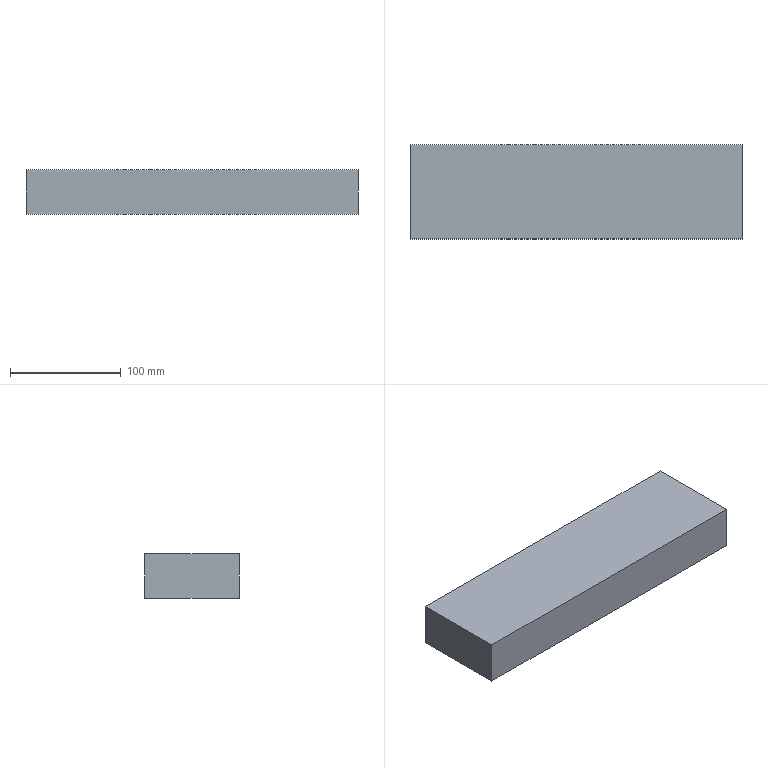Part | NX | features BREP 1 | 1 solid | 6 faces | box 300 x 85 x 40 mm | volume 1020000 mm3 | plane 6
STEP:
#1=CARTESIAN_POINT('',(-150.,42.5,-20.));
#2=VERTEX_POINT('',#1);
#3=CARTESIAN_POINT('',(-150.,-42.5,-20.));
#4=VERTEX_POINT('',#3);
#5=CARTESIAN_POINT('',(-150.,42.5,-20.));
#6=DIRECTION('',(0.,-1.,0.));
#7=VECTOR('',#6,1000.);
#8=LINE('',#5,#7);
#9=EDGE_CURVE('',#2,#4,#8,.T.);
#10=ORIENTED_EDGE('',*,*,#9,.T.);
#11=CARTESIAN_POINT('',(-150.,-42.5,20.));
#12=VERTEX_POINT('',#11);
#13=CARTESIAN_POINT('',(-150.,-42.5,20.));
#14=DIRECTION('',(0.,0.,-1.));
#15=VECTOR('',#14,1000.);
#16=LINE('',#13,#15);
#17=EDGE_CURVE('',#12,#4,#16,.T.);
#18=ORIENTED_EDGE('',*,*,#17,.F.);
#19=CARTESIAN_POINT('',(-150.,42.5,20.));
#20=VERTEX_POINT('',#19);
#21=CARTESIAN_POINT('',(-150.,42.5,20.));
#22=DIRECTION('',(0.,-1.,0.));
#23=VECTOR('',#22,1000.);
#24=LINE('',#21,#23);
#25=EDGE_CURVE('',#20,#12,#24,.T.);
#26=ORIENTED_EDGE('',*,*,#25,.F.);
#27=CARTESIAN_POINT('',(-150.,42.5,20.));
#28=DIRECTION('',(0.,0.,-1.));
#29=VECTOR('',#28,1000.);
#30=LINE('',#27,#29);
#31=EDGE_CURVE('',#20,#2,#30,.T.);
#32=ORIENTED_EDGE('',*,*,#31,.T.);
#33=EDGE_LOOP('',(#10,#18,#26,#32));
#34=FACE_BOUND('',#33,.T.);
#35=CARTESIAN_POINT('',(-150.,42.5,20.));
#36=DIRECTION('',(1.,0.,0.));
#37=DIRECTION('',(0.,0.,1.));
#38=AXIS2_PLACEMENT_3D('',#35,#36,#37);
#39=PLANE('',#38);
#40=ADVANCED_FACE('',(#34),#39,.F.);
#41=CARTESIAN_POINT('',(150.,-42.5,-20.));
#42=VERTEX_POINT('',#41);
#43=CARTESIAN_POINT('',(-150.,-42.5,-20.));
#44=DIRECTION('',(1.,0.,0.));
#45=VECTOR('',#44,1000.);
#46=LINE('',#43,#45);
#47=EDGE_CURVE('',#4,#42,#46,.T.);
#48=ORIENTED_EDGE('',*,*,#47,.T.);
#49=CARTESIAN_POINT('',(150.,-42.5,20.));
#50=VERTEX_POINT('',#49);
#51=CARTESIAN_POINT('',(150.,-42.5,20.));
#52=DIRECTION('',(0.,0.,-1.));
#53=VECTOR('',#52,1000.);
#54=LINE('',#51,#53);
#55=EDGE_CURVE('',#50,#42,#54,.T.);
#56=ORIENTED_EDGE('',*,*,#55,.F.);
#57=CARTESIAN_POINT('',(-150.,-42.5,20.));
#58=DIRECTION('',(1.,0.,0.));
#59=VECTOR('',#58,1000.);
#60=LINE('',#57,#59);
#61=EDGE_CURVE('',#12,#50,#60,.T.);
#62=ORIENTED_EDGE('',*,*,#61,.F.);
#63=ORIENTED_EDGE('',*,*,#17,.T.);
#64=EDGE_LOOP('',(#48,#56,#62,#63));
#65=FACE_BOUND('',#64,.T.);
#66=CARTESIAN_POINT('',(-150.,-42.5,20.));
#67=DIRECTION('',(0.,1.,0.));
#68=DIRECTION('',(0.,0.,-1.));
#69=AXIS2_PLACEMENT_3D('',#66,#67,#68);
#70=PLANE('',#69);
#71=ADVANCED_FACE('',(#65),#70,.F.);
#72=CARTESIAN_POINT('',(150.,42.5,-20.));
#73=VERTEX_POINT('',#72);
#74=CARTESIAN_POINT('',(150.,42.5,-20.));
#75=DIRECTION('',(0.,1.,0.));
#76=VECTOR('',#75,1000.);
#77=LINE('',#74,#76);
#78=EDGE_CURVE('',#42,#73,#77,.T.);
#79=ORIENTED_EDGE('',*,*,#78,.T.);
#80=CARTESIAN_POINT('',(150.,42.5,20.));
#81=VERTEX_POINT('',#80);
#82=CARTESIAN_POINT('',(150.,42.5,20.));
#83=DIRECTION('',(0.,0.,-1.));
#84=VECTOR('',#83,1000.);
#85=LINE('',#82,#84);
#86=EDGE_CURVE('',#81,#73,#85,.T.);
#87=ORIENTED_EDGE('',*,*,#86,.F.);
#88=CARTESIAN_POINT('',(150.,42.5,20.));
#89=DIRECTION('',(0.,1.,0.));
#90=VECTOR('',#89,1000.);
#91=LINE('',#88,#90);
#92=EDGE_CURVE('',#50,#81,#91,.T.);
#93=ORIENTED_EDGE('',*,*,#92,.F.);
#94=ORIENTED_EDGE('',*,*,#55,.T.);
#95=EDGE_LOOP('',(#79,#87,#93,#94));
#96=FACE_BOUND('',#95,.T.);
#97=CARTESIAN_POINT('',(150.,42.5,20.));
#98=DIRECTION('',(-1.,0.,0.));
#99=DIRECTION('',(0.,0.,-1.));
#100=AXIS2_PLACEMENT_3D('',#97,#98,#99);
#101=PLANE('',#100);
#102=ADVANCED_FACE('',(#96),#101,.F.);
#103=CARTESIAN_POINT('',(-150.,42.5,-20.));
#104=DIRECTION('',(-1.,0.,0.));
#105=VECTOR('',#104,1000.);
#106=LINE('',#103,#105);
#107=EDGE_CURVE('',#73,#2,#106,.T.);
#108=ORIENTED_EDGE('',*,*,#107,.T.);
#109=ORIENTED_EDGE('',*,*,#31,.F.);
#110=CARTESIAN_POINT('',(-150.,42.5,20.));
#111=DIRECTION('',(-1.,0.,0.));
#112=VECTOR('',#111,1000.);
#113=LINE('',#110,#112);
#114=EDGE_CURVE('',#81,#20,#113,.T.);
#115=ORIENTED_EDGE('',*,*,#114,.F.);
#116=ORIENTED_EDGE('',*,*,#86,.T.);
#117=EDGE_LOOP('',(#108,#109,#115,#116));
#118=FACE_BOUND('',#117,.T.);
#119=CARTESIAN_POINT('',(-150.,42.5,20.));
#120=DIRECTION('',(0.,-1.,0.));
#121=DIRECTION('',(0.,0.,1.));
#122=AXIS2_PLACEMENT_3D('',#119,#120,#121);
#123=PLANE('',#122);
#124=ADVANCED_FACE('',(#118),#123,.F.);
#125=ORIENTED_EDGE('',*,*,#25,.T.);
#126=ORIENTED_EDGE('',*,*,#61,.T.);
#127=ORIENTED_EDGE('',*,*,#92,.T.);
#128=ORIENTED_EDGE('',*,*,#114,.T.);
#129=EDGE_LOOP('',(#125,#126,#127,#128));
#130=FACE_BOUND('',#129,.T.);
#131=CARTESIAN_POINT('',(-150.,-42.5,20.));
#132=DIRECTION('',(0.,0.,1.));
#133=DIRECTION('',(-1.,0.,0.));
#134=AXIS2_PLACEMENT_3D('',#131,#132,#133);
#135=PLANE('',#134);
#136=ADVANCED_FACE('',(#130),#135,.T.);
#137=ORIENTED_EDGE('',*,*,#9,.F.);
#138=ORIENTED_EDGE('',*,*,#107,.F.);
#139=ORIENTED_EDGE('',*,*,#78,.F.);
#140=ORIENTED_EDGE('',*,*,#47,.F.);
#141=EDGE_LOOP('',(#137,#138,#139,#140));
#142=FACE_BOUND('',#141,.T.);
#143=CARTESIAN_POINT('',(-150.,-42.5,-20.));
#144=DIRECTION('',(0.,0.,1.));
#145=DIRECTION('',(-1.,0.,0.));
#146=AXIS2_PLACEMENT_3D('',#143,#144,#145);
#147=PLANE('',#146);
#148=ADVANCED_FACE('',(#142),#147,.F.);
#149=CLOSED_SHELL('',(#40,#71,#102,#124,#136,#148));
#150=MANIFOLD_SOLID_BREP('',#149);
#151=(LENGTH_UNIT()NAMED_UNIT(*)SI_UNIT(.MILLI.,.METRE.));
#152=UNCERTAINTY_MEASURE_WITH_UNIT(LENGTH_MEASURE(0.00001),#151,'','');
#153=(NAMED_UNIT(*)PLANE_ANGLE_UNIT()SI_UNIT($,.RADIAN.));
#154=(NAMED_UNIT(*)SI_UNIT($,.STERADIAN.)SOLID_ANGLE_UNIT());
#155=(GEOMETRIC_REPRESENTATION_CONTEXT(3)GLOBAL_UNCERTAINTY_ASSIGNED_CONTEXT((#152))GLOBAL_UNIT_ASSIGNED_CONTEXT((#151,#153,#154))REPRESENTATION_CONTEXT('',''));
#156=ADVANCED_BREP_SHAPE_REPRESENTATION('',(#150),#155);